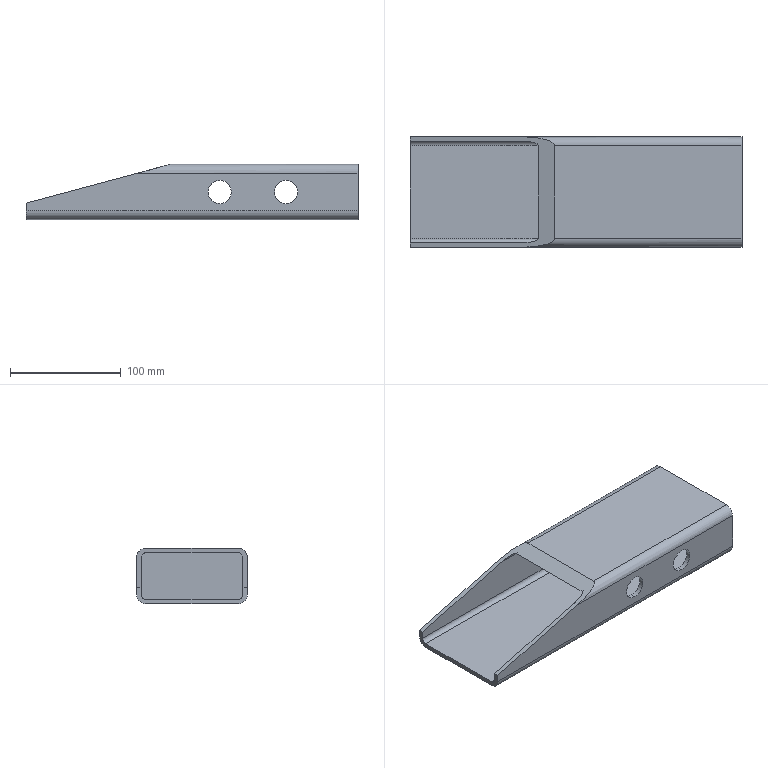Part | SolidWorks | features ICE 2, 3DProfileFeature 1, WeldMemberFeat 1, WeldmentFeature 1 | 2 solids | 37 faces | box 300 x 100 x 50 mm | volume 358178 mm3 | cylinder 20 | plane 17 | commonest cylinder face diameters 8 x8 21 x8 16 x4
STEP:
#1=CARTESIAN_POINT('',(235.,50.,-10.5));
#2=VERTEX_POINT('',#1);
#3=CARTESIAN_POINT('',(235.,50.,10.5));
#4=VERTEX_POINT('',#3);
#5=CARTESIAN_POINT('',(235.,50.,0.));
#6=DIRECTION('',(0.,1.,0.));
#7=DIRECTION('',(0.,0.,-1.));
#8=AXIS2_PLACEMENT_3D('',#5,#6,#7);
#9=CIRCLE('',#8,10.5);
#10=EDGE_CURVE('',#2,#4,#9,.T.);
#11=ORIENTED_EDGE('',*,*,#10,.T.);
#12=CARTESIAN_POINT('',(235.,46.,10.5));
#13=VERTEX_POINT('',#12);
#14=CARTESIAN_POINT('',(235.,185.23,10.5));
#15=DIRECTION('',(0.,-1.,0.));
#16=VECTOR('',#15,1000.);
#17=LINE('',#14,#16);
#18=EDGE_CURVE('',#4,#13,#17,.T.);
#19=ORIENTED_EDGE('',*,*,#18,.T.);
#20=CARTESIAN_POINT('',(235.,46.,-10.5));
#21=VERTEX_POINT('',#20);
#22=CARTESIAN_POINT('',(235.,46.,0.));
#23=DIRECTION('',(0.,-1.,0.));
#24=DIRECTION('',(0.,0.,-1.));
#25=AXIS2_PLACEMENT_3D('',#22,#23,#24);
#26=CIRCLE('',#25,10.5);
#27=EDGE_CURVE('',#13,#21,#26,.T.);
#28=ORIENTED_EDGE('',*,*,#27,.T.);
#29=CARTESIAN_POINT('',(235.,185.23,-10.5));
#30=DIRECTION('',(0.,-1.,0.));
#31=VECTOR('',#30,1000.);
#32=LINE('',#29,#31);
#33=EDGE_CURVE('',#2,#21,#32,.T.);
#34=ORIENTED_EDGE('',*,*,#33,.F.);
#35=EDGE_LOOP('',(#11,#19,#28,#34));
#36=FACE_OUTER_BOUND('',#35,.T.);
#37=CARTESIAN_POINT('',(235.,185.23,0.));
#38=DIRECTION('',(0.,-1.,0.));
#39=DIRECTION('',(0.,0.,-1.));
#40=AXIS2_PLACEMENT_3D('',#37,#38,#39);
#41=CYLINDRICAL_SURFACE('',#40,10.5);
#42=ADVANCED_FACE('',(#36),#41,.F.);
#43=CARTESIAN_POINT('',(175.,50.,-10.5));
#44=VERTEX_POINT('',#43);
#45=CARTESIAN_POINT('',(175.,50.,10.5));
#46=VERTEX_POINT('',#45);
#47=CARTESIAN_POINT('',(175.,50.,0.));
#48=DIRECTION('',(0.,1.,0.));
#49=DIRECTION('',(0.,0.,-1.));
#50=AXIS2_PLACEMENT_3D('',#47,#48,#49);
#51=CIRCLE('',#50,10.5);
#52=EDGE_CURVE('',#44,#46,#51,.T.);
#53=ORIENTED_EDGE('',*,*,#52,.T.);
#54=CARTESIAN_POINT('',(175.,46.,10.5));
#55=VERTEX_POINT('',#54);
#56=CARTESIAN_POINT('',(175.,185.23,10.5));
#57=DIRECTION('',(0.,-1.,0.));
#58=VECTOR('',#57,1000.);
#59=LINE('',#56,#58);
#60=EDGE_CURVE('',#46,#55,#59,.T.);
#61=ORIENTED_EDGE('',*,*,#60,.T.);
#62=CARTESIAN_POINT('',(175.,46.,-10.5));
#63=VERTEX_POINT('',#62);
#64=CARTESIAN_POINT('',(175.,46.,0.));
#65=DIRECTION('',(0.,-1.,0.));
#66=DIRECTION('',(0.,0.,-1.));
#67=AXIS2_PLACEMENT_3D('',#64,#65,#66);
#68=CIRCLE('',#67,10.5);
#69=EDGE_CURVE('',#55,#63,#68,.T.);
#70=ORIENTED_EDGE('',*,*,#69,.T.);
#71=CARTESIAN_POINT('',(175.,185.23,-10.5));
#72=DIRECTION('',(0.,-1.,0.));
#73=VECTOR('',#72,1000.);
#74=LINE('',#71,#73);
#75=EDGE_CURVE('',#44,#63,#74,.T.);
#76=ORIENTED_EDGE('',*,*,#75,.F.);
#77=EDGE_LOOP('',(#53,#61,#70,#76));
#78=FACE_OUTER_BOUND('',#77,.T.);
#79=CARTESIAN_POINT('',(175.,185.23,0.));
#80=DIRECTION('',(0.,-1.,0.));
#81=DIRECTION('',(0.,0.,-1.));
#82=AXIS2_PLACEMENT_3D('',#79,#80,#81);
#83=CYLINDRICAL_SURFACE('',#82,10.5);
#84=ADVANCED_FACE('',(#78),#83,.F.);
#85=CARTESIAN_POINT('',(235.,-46.,-10.5));
#86=VERTEX_POINT('',#85);
#87=CARTESIAN_POINT('',(235.,-46.,10.5));
#88=VERTEX_POINT('',#87);
#89=CARTESIAN_POINT('',(235.,-46.,0.));
#90=DIRECTION('',(0.,1.,0.));
#91=DIRECTION('',(0.,0.,1.));
#92=AXIS2_PLACEMENT_3D('',#89,#90,#91);
#93=CIRCLE('',#92,10.5);
#94=EDGE_CURVE('',#86,#88,#93,.T.);
#95=ORIENTED_EDGE('',*,*,#94,.T.);
#96=CARTESIAN_POINT('',(235.,-50.,10.5));
#97=VERTEX_POINT('',#96);
#98=CARTESIAN_POINT('',(235.,185.23,10.5));
#99=DIRECTION('',(0.,-1.,0.));
#100=VECTOR('',#99,1000.);
#101=LINE('',#98,#100);
#102=EDGE_CURVE('',#88,#97,#101,.T.);
#103=ORIENTED_EDGE('',*,*,#102,.T.);
#104=CARTESIAN_POINT('',(235.,-50.,-10.5));
#105=VERTEX_POINT('',#104);
#106=CARTESIAN_POINT('',(235.,-50.,0.));
#107=DIRECTION('',(0.,-1.,0.));
#108=DIRECTION('',(0.,0.,-1.));
#109=AXIS2_PLACEMENT_3D('',#106,#107,#108);
#110=CIRCLE('',#109,10.5);
#111=EDGE_CURVE('',#97,#105,#110,.T.);
#112=ORIENTED_EDGE('',*,*,#111,.T.);
#113=CARTESIAN_POINT('',(235.,185.23,-10.5));
#114=DIRECTION('',(0.,-1.,0.));
#115=VECTOR('',#114,1000.);
#116=LINE('',#113,#115);
#117=EDGE_CURVE('',#86,#105,#116,.T.);
#118=ORIENTED_EDGE('',*,*,#117,.F.);
#119=EDGE_LOOP('',(#95,#103,#112,#118));
#120=FACE_OUTER_BOUND('',#119,.T.);
#121=CARTESIAN_POINT('',(235.,185.23,0.));
#122=DIRECTION('',(0.,-1.,0.));
#123=DIRECTION('',(0.,0.,-1.));
#124=AXIS2_PLACEMENT_3D('',#121,#122,#123);
#125=CYLINDRICAL_SURFACE('',#124,10.5);
#126=ADVANCED_FACE('',(#120),#125,.F.);
#127=CARTESIAN_POINT('',(175.,-46.,-10.5));
#128=VERTEX_POINT('',#127);
#129=CARTESIAN_POINT('',(175.,-46.,10.5));
#130=VERTEX_POINT('',#129);
#131=CARTESIAN_POINT('',(175.,-46.,0.));
#132=DIRECTION('',(0.,1.,0.));
#133=DIRECTION('',(0.,0.,1.));
#134=AXIS2_PLACEMENT_3D('',#131,#132,#133);
#135=CIRCLE('',#134,10.5);
#136=EDGE_CURVE('',#128,#130,#135,.T.);
#137=ORIENTED_EDGE('',*,*,#136,.T.);
#138=CARTESIAN_POINT('',(175.,-50.,10.5));
#139=VERTEX_POINT('',#138);
#140=CARTESIAN_POINT('',(175.,185.23,10.5));
#141=DIRECTION('',(0.,-1.,0.));
#142=VECTOR('',#141,1000.);
#143=LINE('',#140,#142);
#144=EDGE_CURVE('',#130,#139,#143,.T.);
#145=ORIENTED_EDGE('',*,*,#144,.T.);
#146=CARTESIAN_POINT('',(175.,-50.,-10.5));
#147=VERTEX_POINT('',#146);
#148=CARTESIAN_POINT('',(175.,-50.,0.));
#149=DIRECTION('',(0.,-1.,0.));
#150=DIRECTION('',(0.,0.,-1.));
#151=AXIS2_PLACEMENT_3D('',#148,#149,#150);
#152=CIRCLE('',#151,10.5);
#153=EDGE_CURVE('',#139,#147,#152,.T.);
#154=ORIENTED_EDGE('',*,*,#153,.T.);
#155=CARTESIAN_POINT('',(175.,185.23,-10.5));
#156=DIRECTION('',(0.,-1.,0.));
#157=VECTOR('',#156,1000.);
#158=LINE('',#155,#157);
#159=EDGE_CURVE('',#128,#147,#158,.T.);
#160=ORIENTED_EDGE('',*,*,#159,.F.);
#161=EDGE_LOOP('',(#137,#145,#154,#160));
#162=FACE_OUTER_BOUND('',#161,.T.);
#163=CARTESIAN_POINT('',(175.,185.23,0.));
#164=DIRECTION('',(0.,-1.,0.));
#165=DIRECTION('',(0.,0.,-1.));
#166=AXIS2_PLACEMENT_3D('',#163,#164,#165);
#167=CYLINDRICAL_SURFACE('',#166,10.5);
#168=ADVANCED_FACE('',(#162),#167,.F.);
#169=CARTESIAN_POINT('',(0.,42.,-25.));
#170=VERTEX_POINT('',#169);
#171=CARTESIAN_POINT('',(0.,50.,-17.));
#172=VERTEX_POINT('',#171);
#173=CARTESIAN_POINT('',(0.,42.,-17.));
#174=DIRECTION('',(1.,0.,0.));
#175=DIRECTION('',(0.,0.,-1.));
#176=AXIS2_PLACEMENT_3D('',#173,#174,#175);
#177=CIRCLE('',#176,8.);
#178=EDGE_CURVE('',#170,#172,#177,.T.);
#179=ORIENTED_EDGE('',*,*,#178,.T.);
#180=CARTESIAN_POINT('',(300.,50.,-17.));
#181=VERTEX_POINT('',#180);
#182=CARTESIAN_POINT('',(300.,50.,-17.));
#183=DIRECTION('',(-1.,0.,0.));
#184=VECTOR('',#183,1000.);
#185=LINE('',#182,#184);
#186=EDGE_CURVE('',#181,#172,#185,.T.);
#187=ORIENTED_EDGE('',*,*,#186,.F.);
#188=CARTESIAN_POINT('',(300.,42.,-25.));
#189=VERTEX_POINT('',#188);
#190=CARTESIAN_POINT('',(300.,42.,-17.));
#191=DIRECTION('',(1.,0.,0.));
#192=DIRECTION('',(0.,0.,-1.));
#193=AXIS2_PLACEMENT_3D('',#190,#191,#192);
#194=CIRCLE('',#193,8.);
#195=EDGE_CURVE('',#189,#181,#194,.T.);
#196=ORIENTED_EDGE('',*,*,#195,.F.);
#197=CARTESIAN_POINT('',(300.,42.,-25.));
#198=DIRECTION('',(-1.,0.,0.));
#199=VECTOR('',#198,1000.);
#200=LINE('',#197,#199);
#201=EDGE_CURVE('',#189,#170,#200,.T.);
#202=ORIENTED_EDGE('',*,*,#201,.T.);
#203=EDGE_LOOP('',(#179,#187,#196,#202));
#204=FACE_OUTER_BOUND('',#203,.T.);
#205=CARTESIAN_POINT('',(300.,42.,-17.));
#206=DIRECTION('',(-1.,0.,0.));
#207=DIRECTION('',(0.,0.,1.));
#208=AXIS2_PLACEMENT_3D('',#205,#206,#207);
#209=CYLINDRICAL_SURFACE('',#208,8.);
#210=ADVANCED_FACE('',(#204),#209,.T.);
#211=ORIENTED_EDGE('',*,*,#10,.F.);
#212=CARTESIAN_POINT('',(235.,50.,0.));
#213=DIRECTION('',(0.,1.,0.));
#214=DIRECTION('',(0.,0.,-1.));
#215=AXIS2_PLACEMENT_3D('',#212,#213,#214);
#216=CIRCLE('',#215,10.5);
#217=EDGE_CURVE('',#4,#2,#216,.T.);
#218=ORIENTED_EDGE('',*,*,#217,.F.);
#219=EDGE_LOOP('',(#211,#218));
#220=FACE_BOUND('',#219,.T.);
#221=ORIENTED_EDGE('',*,*,#52,.F.);
#222=CARTESIAN_POINT('',(175.,50.,0.));
#223=DIRECTION('',(0.,1.,0.));
#224=DIRECTION('',(0.,0.,-1.));
#225=AXIS2_PLACEMENT_3D('',#222,#223,#224);
#226=CIRCLE('',#225,10.5);
#227=EDGE_CURVE('',#46,#44,#226,.T.);
#228=ORIENTED_EDGE('',*,*,#227,.F.);
#229=EDGE_LOOP('',(#221,#228));
#230=FACE_BOUND('',#229,.T.);
#231=CARTESIAN_POINT('',(0.,50.,-10.));
#232=VERTEX_POINT('',#231);
#233=CARTESIAN_POINT('',(0.,50.,-17.));
#234=DIRECTION('',(0.,0.,1.));
#235=VECTOR('',#234,1000.);
#236=LINE('',#233,#235);
#237=EDGE_CURVE('',#172,#232,#236,.T.);
#238=ORIENTED_EDGE('',*,*,#237,.T.);
#239=CARTESIAN_POINT('',(100.765,50.,17.));
#240=VERTEX_POINT('',#239);
#241=CARTESIAN_POINT('',(0.,50.,-10.));
#242=DIRECTION('',(-0.9659,0.,-0.2588));
#243=VECTOR('',#242,1000.);
#244=LINE('',#241,#243);
#245=EDGE_CURVE('',#240,#232,#244,.T.);
#246=ORIENTED_EDGE('',*,*,#245,.F.);
#247=CARTESIAN_POINT('',(300.,50.,17.));
#248=VERTEX_POINT('',#247);
#249=CARTESIAN_POINT('',(300.,50.,17.));
#250=DIRECTION('',(-1.,0.,0.));
#251=VECTOR('',#250,1000.);
#252=LINE('',#249,#251);
#253=EDGE_CURVE('',#248,#240,#252,.T.);
#254=ORIENTED_EDGE('',*,*,#253,.F.);
#255=CARTESIAN_POINT('',(300.,50.,-17.));
#256=DIRECTION('',(0.,0.,1.));
#257=VECTOR('',#256,1000.);
#258=LINE('',#255,#257);
#259=EDGE_CURVE('',#181,#248,#258,.T.);
#260=ORIENTED_EDGE('',*,*,#259,.F.);
#261=ORIENTED_EDGE('',*,*,#186,.T.);
#262=EDGE_LOOP('',(#238,#246,#254,#260,#261));
#263=FACE_OUTER_BOUND('',#262,.T.);
#264=CARTESIAN_POINT('',(300.,50.,-17.));
#265=DIRECTION('',(0.,-1.,0.));
#266=DIRECTION('',(0.,0.,-1.));
#267=AXIS2_PLACEMENT_3D('',#264,#265,#266);
#268=PLANE('',#267);
#269=ADVANCED_FACE('',(#220,#230,#263),#268,.F.);
#270=ORIENTED_EDGE('',*,*,#253,.T.);
#271=CARTESIAN_POINT('',(130.622,42.,25.));
#272=VERTEX_POINT('',#271);
#273=CARTESIAN_POINT('',(100.765,50.,17.));
#274=CARTESIAN_POINT('',(118.255,50.,21.686));
#275=CARTESIAN_POINT('',(130.622,46.686,25.));
#276=CARTESIAN_POINT('',(130.622,42.,25.));
#277=(BOUNDED_CURVE()B_SPLINE_CURVE(3,(#273,#274,#275,#276),.UNSPECIFIED.,.F.,.F.)B_SPLINE_CURVE_WITH_KNOTS((4,4),(1.571,3.142),.UNSPECIFIED.)CURVE()GEOMETRIC_REPRESENTATION_ITEM()RATIONAL_B_SPLINE_CURVE((1.,0.8047,0.8047,1.))REPRESENTATION_ITEM(''));
#278=EDGE_CURVE('',#240,#272,#277,.T.);
#279=ORIENTED_EDGE('',*,*,#278,.T.);
#280=CARTESIAN_POINT('',(300.,42.,25.));
#281=VERTEX_POINT('',#280);
#282=CARTESIAN_POINT('',(300.,42.,25.));
#283=DIRECTION('',(-1.,0.,0.));
#284=VECTOR('',#283,1000.);
#285=LINE('',#282,#284);
#286=EDGE_CURVE('',#281,#272,#285,.T.);
#287=ORIENTED_EDGE('',*,*,#286,.F.);
#288=CARTESIAN_POINT('',(300.,42.,17.));
#289=DIRECTION('',(1.,0.,0.));
#290=DIRECTION('',(0.,0.,-1.));
#291=AXIS2_PLACEMENT_3D('',#288,#289,#290);
#292=CIRCLE('',#291,8.);
#293=EDGE_CURVE('',#248,#281,#292,.T.);
#294=ORIENTED_EDGE('',*,*,#293,.F.);
#295=EDGE_LOOP('',(#270,#279,#287,#294));
#296=FACE_OUTER_BOUND('',#295,.T.);
#297=CARTESIAN_POINT('',(300.,42.,17.));
#298=DIRECTION('',(-1.,0.,0.));
#299=DIRECTION('',(0.,0.,1.));
#300=AXIS2_PLACEMENT_3D('',#297,#298,#299);
#301=CYLINDRICAL_SURFACE('',#300,8.);
#302=ADVANCED_FACE('',(#296),#301,.T.);
#303=ORIENTED_EDGE('',*,*,#286,.T.);
#304=CARTESIAN_POINT('',(130.622,-42.,25.));
#305=VERTEX_POINT('',#304);
#306=CARTESIAN_POINT('',(130.622,185.23,25.));
#307=DIRECTION('',(0.,-1.,0.));
#308=VECTOR('',#307,1000.);
#309=LINE('',#306,#308);
#310=EDGE_CURVE('',#272,#305,#309,.T.);
#311=ORIENTED_EDGE('',*,*,#310,.T.);
#312=CARTESIAN_POINT('',(300.,-42.,25.));
#313=VERTEX_POINT('',#312);
#314=CARTESIAN_POINT('',(300.,-42.,25.));
#315=DIRECTION('',(-1.,0.,0.));
#316=VECTOR('',#315,1000.);
#317=LINE('',#314,#316);
#318=EDGE_CURVE('',#313,#305,#317,.T.);
#319=ORIENTED_EDGE('',*,*,#318,.F.);
#320=CARTESIAN_POINT('',(300.,-42.,25.));
#321=DIRECTION('',(0.,-1.,0.));
#322=VECTOR('',#321,1000.);
#323=LINE('',#320,#322);
#324=EDGE_CURVE('',#281,#313,#323,.T.);
#325=ORIENTED_EDGE('',*,*,#324,.F.);
#326=EDGE_LOOP('',(#303,#311,#319,#325));
#327=FACE_OUTER_BOUND('',#326,.T.);
#328=CARTESIAN_POINT('',(300.,-42.,25.));
#329=DIRECTION('',(0.,0.,-1.));
#330=DIRECTION('',(-1.,0.,0.));
#331=AXIS2_PLACEMENT_3D('',#328,#329,#330);
#332=PLANE('',#331);
#333=ADVANCED_FACE('',(#327),#332,.F.);
#334=ORIENTED_EDGE('',*,*,#318,.T.);
#335=CARTESIAN_POINT('',(100.765,-50.,17.));
#336=VERTEX_POINT('',#335);
#337=CARTESIAN_POINT('',(130.622,-42.,25.));
#338=CARTESIAN_POINT('',(130.622,-46.686,25.));
#339=CARTESIAN_POINT('',(118.255,-50.,21.686));
#340=CARTESIAN_POINT('',(100.765,-50.,17.));
#341=(BOUNDED_CURVE()B_SPLINE_CURVE(3,(#337,#338,#339,#340),.UNSPECIFIED.,.F.,.F.)B_SPLINE_CURVE_WITH_KNOTS((4,4),(3.142,4.712),.UNSPECIFIED.)CURVE()GEOMETRIC_REPRESENTATION_ITEM()RATIONAL_B_SPLINE_CURVE((1.,0.8047,0.8047,1.))REPRESENTATION_ITEM(''));
#342=EDGE_CURVE('',#305,#336,#341,.T.);
#343=ORIENTED_EDGE('',*,*,#342,.T.);
#344=CARTESIAN_POINT('',(300.,-50.,17.));
#345=VERTEX_POINT('',#344);
#346=CARTESIAN_POINT('',(300.,-50.,17.));
#347=DIRECTION('',(-1.,0.,0.));
#348=VECTOR('',#347,1000.);
#349=LINE('',#346,#348);
#350=EDGE_CURVE('',#345,#336,#349,.T.);
#351=ORIENTED_EDGE('',*,*,#350,.F.);
#352=CARTESIAN_POINT('',(300.,-42.,17.));
#353=DIRECTION('',(1.,0.,0.));
#354=DIRECTION('',(0.,0.,-1.));
#355=AXIS2_PLACEMENT_3D('',#352,#353,#354);
#356=CIRCLE('',#355,8.);
#357=EDGE_CURVE('',#313,#345,#356,.T.);
#358=ORIENTED_EDGE('',*,*,#357,.F.);
#359=EDGE_LOOP('',(#334,#343,#351,#358));
#360=FACE_OUTER_BOUND('',#359,.T.);
#361=CARTESIAN_POINT('',(300.,-42.,17.));
#362=DIRECTION('',(-1.,0.,0.));
#363=DIRECTION('',(0.,0.,1.));
#364=AXIS2_PLACEMENT_3D('',#361,#362,#363);
#365=CYLINDRICAL_SURFACE('',#364,8.);
#366=ADVANCED_FACE('',(#360),#365,.T.);
#367=CARTESIAN_POINT('',(235.,-50.,0.));
#368=DIRECTION('',(0.,-1.,0.));
#369=DIRECTION('',(0.,0.,-1.));
#370=AXIS2_PLACEMENT_3D('',#367,#368,#369);
#371=CIRCLE('',#370,10.5);
#372=EDGE_CURVE('',#105,#97,#371,.T.);
#373=ORIENTED_EDGE('',*,*,#372,.F.);
#374=ORIENTED_EDGE('',*,*,#111,.F.);
#375=EDGE_LOOP('',(#373,#374));
#376=FACE_BOUND('',#375,.T.);
#377=CARTESIAN_POINT('',(175.,-50.,0.));
#378=DIRECTION('',(0.,-1.,0.));
#379=DIRECTION('',(0.,0.,-1.));
#380=AXIS2_PLACEMENT_3D('',#377,#378,#379);
#381=CIRCLE('',#380,10.5);
#382=EDGE_CURVE('',#147,#139,#381,.T.);
#383=ORIENTED_EDGE('',*,*,#382,.F.);
#384=ORIENTED_EDGE('',*,*,#153,.F.);
#385=EDGE_LOOP('',(#383,#384));
#386=FACE_BOUND('',#385,.T.);
#387=ORIENTED_EDGE('',*,*,#350,.T.);
#388=CARTESIAN_POINT('',(0.,-50.,-10.));
#389=VERTEX_POINT('',#388);
#390=CARTESIAN_POINT('',(0.,-50.,-10.));
#391=DIRECTION('',(0.9659,0.,0.2588));
#392=VECTOR('',#391,1000.);
#393=LINE('',#390,#392);
#394=EDGE_CURVE('',#389,#336,#393,.T.);
#395=ORIENTED_EDGE('',*,*,#394,.F.);
#396=CARTESIAN_POINT('',(0.,-50.,-17.));
#397=VERTEX_POINT('',#396);
#398=CARTESIAN_POINT('',(0.,-50.,17.));
#399=DIRECTION('',(0.,0.,-1.));
#400=VECTOR('',#399,1000.);
#401=LINE('',#398,#400);
#402=EDGE_CURVE('',#389,#397,#401,.T.);
#403=ORIENTED_EDGE('',*,*,#402,.T.);
#404=CARTESIAN_POINT('',(300.,-50.,-17.));
#405=VERTEX_POINT('',#404);
#406=CARTESIAN_POINT('',(300.,-50.,-17.));
#407=DIRECTION('',(-1.,0.,0.));
#408=VECTOR('',#407,1000.);
#409=LINE('',#406,#408);
#410=EDGE_CURVE('',#405,#397,#409,.T.);
#411=ORIENTED_EDGE('',*,*,#410,.F.);
#412=CARTESIAN_POINT('',(300.,-50.,17.));
#413=DIRECTION('',(0.,0.,-1.));
#414=VECTOR('',#413,1000.);
#415=LINE('',#412,#414);
#416=EDGE_CURVE('',#345,#405,#415,.T.);
#417=ORIENTED_EDGE('',*,*,#416,.F.);
#418=EDGE_LOOP('',(#387,#395,#403,#411,#417));
#419=FACE_OUTER_BOUND('',#418,.T.);
#420=CARTESIAN_POINT('',(300.,-50.,17.));
#421=DIRECTION('',(0.,1.,0.));
#422=DIRECTION('',(0.,0.,1.));
#423=AXIS2_PLACEMENT_3D('',#420,#421,#422);
#424=PLANE('',#423);
#425=ADVANCED_FACE('',(#376,#386,#419),#424,.F.);
#426=CARTESIAN_POINT('',(0.,-42.,-25.));
#427=VERTEX_POINT('',#426);
#428=CARTESIAN_POINT('',(0.,-42.,-17.));
#429=DIRECTION('',(1.,0.,0.));
#430=DIRECTION('',(0.,0.,-1.));
#431=AXIS2_PLACEMENT_3D('',#428,#429,#430);
#432=CIRCLE('',#431,8.);
#433=EDGE_CURVE('',#397,#427,#432,.T.);
#434=ORIENTED_EDGE('',*,*,#433,.T.);
#435=CARTESIAN_POINT('',(300.,-42.,-25.));
#436=VERTEX_POINT('',#435);
#437=CARTESIAN_POINT('',(300.,-42.,-25.));
#438=DIRECTION('',(-1.,0.,0.));
#439=VECTOR('',#438,1000.);
#440=LINE('',#437,#439);
#441=EDGE_CURVE('',#436,#427,#440,.T.);
#442=ORIENTED_EDGE('',*,*,#441,.F.);
#443=CARTESIAN_POINT('',(300.,-42.,-17.));
#444=DIRECTION('',(1.,0.,0.));
#445=DIRECTION('',(0.,0.,-1.));
#446=AXIS2_PLACEMENT_3D('',#443,#444,#445);
#447=CIRCLE('',#446,8.);
#448=EDGE_CURVE('',#405,#436,#447,.T.);
#449=ORIENTED_EDGE('',*,*,#448,.F.);
#450=ORIENTED_EDGE('',*,*,#410,.T.);
#451=EDGE_LOOP('',(#434,#442,#449,#450));
#452=FACE_OUTER_BOUND('',#451,.T.);
#453=CARTESIAN_POINT('',(300.,-42.,-17.));
#454=DIRECTION('',(-1.,0.,0.));
#455=DIRECTION('',(0.,0.,1.));
#456=AXIS2_PLACEMENT_3D('',#453,#454,#455);
#457=CYLINDRICAL_SURFACE('',#456,8.);
#458=ADVANCED_FACE('',(#452),#457,.T.);
#459=CARTESIAN_POINT('',(100.765,46.,17.));
#460=VERTEX_POINT('',#459);
#461=CARTESIAN_POINT('',(115.694,42.,21.));
#462=VERTEX_POINT('',#461);
#463=CARTESIAN_POINT('',(100.765,46.,17.));
#464=CARTESIAN_POINT('',(109.51,46.,19.343));
#465=CARTESIAN_POINT('',(115.694,44.343,21.));
#466=CARTESIAN_POINT('',(115.694,42.,21.));
#467=(BOUNDED_CURVE()B_SPLINE_CURVE(3,(#463,#464,#465,#466),.UNSPECIFIED.,.F.,.F.)B_SPLINE_CURVE_WITH_KNOTS((4,4),(1.571,3.142),.UNSPECIFIED.)CURVE()GEOMETRIC_REPRESENTATION_ITEM()RATIONAL_B_SPLINE_CURVE((1.,0.8047,0.8047,1.))REPRESENTATION_ITEM(''));
#468=EDGE_CURVE('',#460,#462,#467,.T.);
#469=ORIENTED_EDGE('',*,*,#468,.F.);
#470=CARTESIAN_POINT('',(300.,46.,17.));
#471=VERTEX_POINT('',#470);
#472=CARTESIAN_POINT('',(300.,46.,17.));
#473=DIRECTION('',(-1.,0.,0.));
#474=VECTOR('',#473,1000.);
#475=LINE('',#472,#474);
#476=EDGE_CURVE('',#471,#460,#475,.T.);
#477=ORIENTED_EDGE('',*,*,#476,.F.);
#478=CARTESIAN_POINT('',(300.,42.,21.));
#479=VERTEX_POINT('',#478);
#480=CARTESIAN_POINT('',(300.,42.,17.));
#481=DIRECTION('',(1.,0.,0.));
#482=DIRECTION('',(0.,0.,-1.));
#483=AXIS2_PLACEMENT_3D('',#480,#481,#482);
#484=CIRCLE('',#483,4.);
#485=EDGE_CURVE('',#471,#479,#484,.T.);
#486=ORIENTED_EDGE('',*,*,#485,.T.);
#487=CARTESIAN_POINT('',(300.,42.,21.));
#488=DIRECTION('',(-1.,0.,0.));
#489=VECTOR('',#488,1000.);
#490=LINE('',#487,#489);
#491=EDGE_CURVE('',#479,#462,#490,.T.);
#492=ORIENTED_EDGE('',*,*,#491,.T.);
#493=EDGE_LOOP('',(#469,#477,#486,#492));
#494=FACE_OUTER_BOUND('',#493,.T.);
#495=CARTESIAN_POINT('',(300.,42.,17.));
#496=DIRECTION('',(-1.,0.,0.));
#497=DIRECTION('',(0.,0.,1.));
#498=AXIS2_PLACEMENT_3D('',#495,#496,#497);
#499=CYLINDRICAL_SURFACE('',#498,4.);
#500=ADVANCED_FACE('',(#494),#499,.F.);
#501=CARTESIAN_POINT('',(235.,46.,0.));
#502=DIRECTION('',(0.,-1.,0.));
#503=DIRECTION('',(0.,0.,-1.));
#504=AXIS2_PLACEMENT_3D('',#501,#502,#503);
#505=CIRCLE('',#504,10.5);
#506=EDGE_CURVE('',#21,#13,#505,.T.);
#507=ORIENTED_EDGE('',*,*,#506,.F.);
#508=ORIENTED_EDGE('',*,*,#27,.F.);
#509=EDGE_LOOP('',(#507,#508));
#510=FACE_BOUND('',#509,.T.);
#511=CARTESIAN_POINT('',(175.,46.,0.));
#512=DIRECTION('',(0.,-1.,0.));
#513=DIRECTION('',(0.,0.,-1.));
#514=AXIS2_PLACEMENT_3D('',#511,#512,#513);
#515=CIRCLE('',#514,10.5);
#516=EDGE_CURVE('',#63,#55,#515,.T.);
#517=ORIENTED_EDGE('',*,*,#516,.F.);
#518=ORIENTED_EDGE('',*,*,#69,.F.);
#519=EDGE_LOOP('',(#517,#518));
#520=FACE_BOUND('',#519,.T.);
#521=CARTESIAN_POINT('',(0.,46.,-10.));
#522=VERTEX_POINT('',#521);
#523=CARTESIAN_POINT('',(278.154,46.,64.531));
#524=DIRECTION('',(0.9659,0.,0.2588));
#525=VECTOR('',#524,1000.);
#526=LINE('',#523,#525);
#527=EDGE_CURVE('',#522,#460,#526,.T.);
#528=ORIENTED_EDGE('',*,*,#527,.F.);
#529=CARTESIAN_POINT('',(0.,46.,-17.));
#530=VERTEX_POINT('',#529);
#531=CARTESIAN_POINT('',(0.,46.,-17.));
#532=DIRECTION('',(0.,0.,1.));
#533=VECTOR('',#532,1000.);
#534=LINE('',#531,#533);
#535=EDGE_CURVE('',#530,#522,#534,.T.);
#536=ORIENTED_EDGE('',*,*,#535,.F.);
#537=CARTESIAN_POINT('',(300.,46.,-17.));
#538=VERTEX_POINT('',#537);
#539=CARTESIAN_POINT('',(300.,46.,-17.));
#540=DIRECTION('',(-1.,0.,0.));
#541=VECTOR('',#540,1000.);
#542=LINE('',#539,#541);
#543=EDGE_CURVE('',#538,#530,#542,.T.);
#544=ORIENTED_EDGE('',*,*,#543,.F.);
#545=CARTESIAN_POINT('',(300.,46.,-17.));
#546=DIRECTION('',(0.,0.,1.));
#547=VECTOR('',#546,1000.);
#548=LINE('',#545,#547);
#549=EDGE_CURVE('',#538,#471,#548,.T.);
#550=ORIENTED_EDGE('',*,*,#549,.T.);
#551=ORIENTED_EDGE('',*,*,#476,.T.);
#552=EDGE_LOOP('',(#528,#536,#544,#550,#551));
#553=FACE_OUTER_BOUND('',#552,.T.);
#554=CARTESIAN_POINT('',(300.,46.,-17.));
#555=DIRECTION('',(0.,-1.,0.));
#556=DIRECTION('',(0.,0.,-1.));
#557=AXIS2_PLACEMENT_3D('',#554,#555,#556);
#558=PLANE('',#557);
#559=ADVANCED_FACE('',(#510,#520,#553),#558,.T.);
#560=CARTESIAN_POINT('',(0.,42.,-21.));
#561=VERTEX_POINT('',#560);
#562=CARTESIAN_POINT('',(0.,42.,-17.));
#563=DIRECTION('',(1.,0.,0.));
#564=DIRECTION('',(0.,0.,-1.));
#565=AXIS2_PLACEMENT_3D('',#562,#563,#564);
#566=CIRCLE('',#565,4.);
#567=EDGE_CURVE('',#561,#530,#566,.T.);
#568=ORIENTED_EDGE('',*,*,#567,.F.);
#569=CARTESIAN_POINT('',(300.,42.,-21.));
#570=VERTEX_POINT('',#569);
#571=CARTESIAN_POINT('',(300.,42.,-21.));
#572=DIRECTION('',(-1.,0.,0.));
#573=VECTOR('',#572,1000.);
#574=LINE('',#571,#573);
#575=EDGE_CURVE('',#570,#561,#574,.T.);
#576=ORIENTED_EDGE('',*,*,#575,.F.);
#577=CARTESIAN_POINT('',(300.,42.,-17.));
#578=DIRECTION('',(1.,0.,0.));
#579=DIRECTION('',(0.,0.,-1.));
#580=AXIS2_PLACEMENT_3D('',#577,#578,#579);
#581=CIRCLE('',#580,4.);
#582=EDGE_CURVE('',#570,#538,#581,.T.);
#583=ORIENTED_EDGE('',*,*,#582,.T.);
#584=ORIENTED_EDGE('',*,*,#543,.T.);
#585=EDGE_LOOP('',(#568,#576,#583,#584));
#586=FACE_OUTER_BOUND('',#585,.T.);
#587=CARTESIAN_POINT('',(300.,42.,-17.));
#588=DIRECTION('',(-1.,0.,0.));
#589=DIRECTION('',(0.,0.,1.));
#590=AXIS2_PLACEMENT_3D('',#587,#588,#589);
#591=CYLINDRICAL_SURFACE('',#590,4.);
#592=ADVANCED_FACE('',(#586),#591,.F.);
#593=CARTESIAN_POINT('',(0.,-42.,-21.));
#594=VERTEX_POINT('',#593);
#595=CARTESIAN_POINT('',(0.,42.,-21.));
#596=DIRECTION('',(0.,1.,0.));
#597=VECTOR('',#596,1000.);
#598=LINE('',#595,#597);
#599=EDGE_CURVE('',#594,#561,#598,.T.);
#600=ORIENTED_EDGE('',*,*,#599,.F.);
#601=CARTESIAN_POINT('',(300.,-42.,-21.));
#602=VERTEX_POINT('',#601);
#603=CARTESIAN_POINT('',(300.,-42.,-21.));
#604=DIRECTION('',(-1.,0.,0.));
#605=VECTOR('',#604,1000.);
#606=LINE('',#603,#605);
#607=EDGE_CURVE('',#602,#594,#606,.T.);
#608=ORIENTED_EDGE('',*,*,#607,.F.);
#609=CARTESIAN_POINT('',(300.,42.,-21.));
#610=DIRECTION('',(0.,1.,0.));
#611=VECTOR('',#610,1000.);
#612=LINE('',#609,#611);
#613=EDGE_CURVE('',#602,#570,#612,.T.);
#614=ORIENTED_EDGE('',*,*,#613,.T.);
#615=ORIENTED_EDGE('',*,*,#575,.T.);
#616=EDGE_LOOP('',(#600,#608,#614,#615));
#617=FACE_OUTER_BOUND('',#616,.T.);
#618=CARTESIAN_POINT('',(300.,42.,-21.));
#619=DIRECTION('',(0.,0.,1.));
#620=DIRECTION('',(1.,0.,0.));
#621=AXIS2_PLACEMENT_3D('',#618,#619,#620);
#622=PLANE('',#621);
#623=ADVANCED_FACE('',(#617),#622,.T.);
#624=CARTESIAN_POINT('',(0.,-46.,-17.));
#625=VERTEX_POINT('',#624);
#626=CARTESIAN_POINT('',(0.,-42.,-17.));
#627=DIRECTION('',(1.,0.,0.));
#628=DIRECTION('',(0.,0.,-1.));
#629=AXIS2_PLACEMENT_3D('',#626,#627,#628);
#630=CIRCLE('',#629,4.);
#631=EDGE_CURVE('',#625,#594,#630,.T.);
#632=ORIENTED_EDGE('',*,*,#631,.F.);
#633=CARTESIAN_POINT('',(300.,-46.,-17.));
#634=VERTEX_POINT('',#633);
#635=CARTESIAN_POINT('',(300.,-46.,-17.));
#636=DIRECTION('',(-1.,0.,0.));
#637=VECTOR('',#636,1000.);
#638=LINE('',#635,#637);
#639=EDGE_CURVE('',#634,#625,#638,.T.);
#640=ORIENTED_EDGE('',*,*,#639,.F.);
#641=CARTESIAN_POINT('',(300.,-42.,-17.));
#642=DIRECTION('',(1.,0.,0.));
#643=DIRECTION('',(0.,0.,-1.));
#644=AXIS2_PLACEMENT_3D('',#641,#642,#643);
#645=CIRCLE('',#644,4.);
#646=EDGE_CURVE('',#634,#602,#645,.T.);
#647=ORIENTED_EDGE('',*,*,#646,.T.);
#648=ORIENTED_EDGE('',*,*,#607,.T.);
#649=EDGE_LOOP('',(#632,#640,#647,#648));
#650=FACE_OUTER_BOUND('',#649,.T.);
#651=CARTESIAN_POINT('',(300.,-42.,-17.));
#652=DIRECTION('',(-1.,0.,0.));
#653=DIRECTION('',(0.,0.,1.));
#654=AXIS2_PLACEMENT_3D('',#651,#652,#653);
#655=CYLINDRICAL_SURFACE('',#654,4.);
#656=ADVANCED_FACE('',(#650),#655,.F.);
#657=ORIENTED_EDGE('',*,*,#94,.F.);
#658=CARTESIAN_POINT('',(235.,-46.,0.));
#659=DIRECTION('',(0.,1.,0.));
#660=DIRECTION('',(0.,0.,1.));
#661=AXIS2_PLACEMENT_3D('',#658,#659,#660);
#662=CIRCLE('',#661,10.5);
#663=EDGE_CURVE('',#88,#86,#662,.T.);
#664=ORIENTED_EDGE('',*,*,#663,.F.);
#665=EDGE_LOOP('',(#657,#664));
#666=FACE_BOUND('',#665,.T.);
#667=ORIENTED_EDGE('',*,*,#136,.F.);
#668=CARTESIAN_POINT('',(175.,-46.,0.));
#669=DIRECTION('',(0.,1.,0.));
#670=DIRECTION('',(0.,0.,1.));
#671=AXIS2_PLACEMENT_3D('',#668,#669,#670);
#672=CIRCLE('',#671,10.5);
#673=EDGE_CURVE('',#130,#128,#672,.T.);
#674=ORIENTED_EDGE('',*,*,#673,.F.);
#675=EDGE_LOOP('',(#667,#674));
#676=FACE_BOUND('',#675,.T.);
#677=CARTESIAN_POINT('',(100.765,-46.,17.));
#678=VERTEX_POINT('',#677);
#679=CARTESIAN_POINT('',(0.,-46.,-10.));
#680=VERTEX_POINT('',#679);
#681=CARTESIAN_POINT('',(286.654,-46.,66.809));
#682=DIRECTION('',(-0.9659,0.,-0.2588));
#683=VECTOR('',#682,1000.);
#684=LINE('',#681,#683);
#685=EDGE_CURVE('',#678,#680,#684,.T.);
#686=ORIENTED_EDGE('',*,*,#685,.F.);
#687=CARTESIAN_POINT('',(300.,-46.,17.));
#688=VERTEX_POINT('',#687);
#689=CARTESIAN_POINT('',(300.,-46.,17.));
#690=DIRECTION('',(-1.,0.,0.));
#691=VECTOR('',#690,1000.);
#692=LINE('',#689,#691);
#693=EDGE_CURVE('',#688,#678,#692,.T.);
#694=ORIENTED_EDGE('',*,*,#693,.F.);
#695=CARTESIAN_POINT('',(300.,-46.,17.));
#696=DIRECTION('',(0.,0.,-1.));
#697=VECTOR('',#696,1000.);
#698=LINE('',#695,#697);
#699=EDGE_CURVE('',#688,#634,#698,.T.);
#700=ORIENTED_EDGE('',*,*,#699,.T.);
#701=ORIENTED_EDGE('',*,*,#639,.T.);
#702=CARTESIAN_POINT('',(0.,-46.,17.));
#703=DIRECTION('',(0.,0.,-1.));
#704=VECTOR('',#703,1000.);
#705=LINE('',#702,#704);
#706=EDGE_CURVE('',#680,#625,#705,.T.);
#707=ORIENTED_EDGE('',*,*,#706,.F.);
#708=EDGE_LOOP('',(#686,#694,#700,#701,#707));
#709=FACE_OUTER_BOUND('',#708,.T.);
#710=CARTESIAN_POINT('',(300.,-46.,17.));
#711=DIRECTION('',(0.,1.,0.));
#712=DIRECTION('',(0.,0.,1.));
#713=AXIS2_PLACEMENT_3D('',#710,#711,#712);
#714=PLANE('',#713);
#715=ADVANCED_FACE('',(#666,#676,#709),#714,.T.);
#716=CARTESIAN_POINT('',(115.694,-42.,21.));
#717=VERTEX_POINT('',#716);
#718=CARTESIAN_POINT('',(115.694,-42.,21.));
#719=CARTESIAN_POINT('',(115.694,-44.343,21.));
#720=CARTESIAN_POINT('',(109.51,-46.,19.343));
#721=CARTESIAN_POINT('',(100.765,-46.,17.));
#722=(BOUNDED_CURVE()B_SPLINE_CURVE(3,(#718,#719,#720,#721),.UNSPECIFIED.,.F.,.F.)B_SPLINE_CURVE_WITH_KNOTS((4,4),(3.142,4.712),.UNSPECIFIED.)CURVE()GEOMETRIC_REPRESENTATION_ITEM()RATIONAL_B_SPLINE_CURVE((1.,0.8047,0.8047,1.))REPRESENTATION_ITEM(''));
#723=EDGE_CURVE('',#717,#678,#722,.T.);
#724=ORIENTED_EDGE('',*,*,#723,.F.);
#725=CARTESIAN_POINT('',(300.,-42.,21.));
#726=VERTEX_POINT('',#725);
#727=CARTESIAN_POINT('',(300.,-42.,21.));
#728=DIRECTION('',(-1.,0.,0.));
#729=VECTOR('',#728,1000.);
#730=LINE('',#727,#729);
#731=EDGE_CURVE('',#726,#717,#730,.T.);
#732=ORIENTED_EDGE('',*,*,#731,.F.);
#733=CARTESIAN_POINT('',(300.,-42.,17.));
#734=DIRECTION('',(1.,0.,0.));
#735=DIRECTION('',(0.,0.,-1.));
#736=AXIS2_PLACEMENT_3D('',#733,#734,#735);
#737=CIRCLE('',#736,4.);
#738=EDGE_CURVE('',#726,#688,#737,.T.);
#739=ORIENTED_EDGE('',*,*,#738,.T.);
#740=ORIENTED_EDGE('',*,*,#693,.T.);
#741=EDGE_LOOP('',(#724,#732,#739,#740));
#742=FACE_OUTER_BOUND('',#741,.T.);
#743=CARTESIAN_POINT('',(300.,-42.,17.));
#744=DIRECTION('',(-1.,0.,0.));
#745=DIRECTION('',(0.,0.,1.));
#746=AXIS2_PLACEMENT_3D('',#743,#744,#745);
#747=CYLINDRICAL_SURFACE('',#746,4.);
#748=ADVANCED_FACE('',(#742),#747,.F.);
#749=CARTESIAN_POINT('',(115.694,-42.,21.));
#750=DIRECTION('',(0.,-1.,0.));
#751=VECTOR('',#750,1000.);
#752=LINE('',#749,#751);
#753=EDGE_CURVE('',#462,#717,#752,.T.);
#754=ORIENTED_EDGE('',*,*,#753,.F.);
#755=ORIENTED_EDGE('',*,*,#491,.F.);
#756=CARTESIAN_POINT('',(300.,-42.,21.));
#757=DIRECTION('',(0.,-1.,0.));
#758=VECTOR('',#757,1000.);
#759=LINE('',#756,#758);
#760=EDGE_CURVE('',#479,#726,#759,.T.);
#761=ORIENTED_EDGE('',*,*,#760,.T.);
#762=ORIENTED_EDGE('',*,*,#731,.T.);
#763=EDGE_LOOP('',(#754,#755,#761,#762));
#764=FACE_OUTER_BOUND('',#763,.T.);
#765=CARTESIAN_POINT('',(300.,-42.,21.));
#766=DIRECTION('',(0.,0.,-1.));
#767=DIRECTION('',(-1.,0.,0.));
#768=AXIS2_PLACEMENT_3D('',#765,#766,#767);
#769=PLANE('',#768);
#770=ADVANCED_FACE('',(#764),#769,.T.);
#771=CARTESIAN_POINT('',(0.,42.,-25.));
#772=DIRECTION('',(0.,1.,0.));
#773=VECTOR('',#772,1000.);
#774=LINE('',#771,#773);
#775=EDGE_CURVE('',#427,#170,#774,.T.);
#776=ORIENTED_EDGE('',*,*,#775,.T.);
#777=ORIENTED_EDGE('',*,*,#201,.F.);
#778=CARTESIAN_POINT('',(300.,42.,-25.));
#779=DIRECTION('',(0.,1.,0.));
#780=VECTOR('',#779,1000.);
#781=LINE('',#778,#780);
#782=EDGE_CURVE('',#436,#189,#781,.T.);
#783=ORIENTED_EDGE('',*,*,#782,.F.);
#784=ORIENTED_EDGE('',*,*,#441,.T.);
#785=EDGE_LOOP('',(#776,#777,#783,#784));
#786=FACE_OUTER_BOUND('',#785,.T.);
#787=CARTESIAN_POINT('',(300.,42.,-25.));
#788=DIRECTION('',(0.,0.,1.));
#789=DIRECTION('',(1.,0.,0.));
#790=AXIS2_PLACEMENT_3D('',#787,#788,#789);
#791=PLANE('',#790);
#792=ADVANCED_FACE('',(#786),#791,.F.);
#793=ORIENTED_EDGE('',*,*,#485,.F.);
#794=ORIENTED_EDGE('',*,*,#549,.F.);
#795=ORIENTED_EDGE('',*,*,#582,.F.);
#796=ORIENTED_EDGE('',*,*,#613,.F.);
#797=ORIENTED_EDGE('',*,*,#646,.F.);
#798=ORIENTED_EDGE('',*,*,#699,.F.);
#799=ORIENTED_EDGE('',*,*,#738,.F.);
#800=ORIENTED_EDGE('',*,*,#760,.F.);
#801=EDGE_LOOP('',(#793,#794,#795,#796,#797,#798,#799,#800));
#802=FACE_BOUND('',#801,.T.);
#803=ORIENTED_EDGE('',*,*,#195,.T.);
#804=ORIENTED_EDGE('',*,*,#259,.T.);
#805=ORIENTED_EDGE('',*,*,#293,.T.);
#806=ORIENTED_EDGE('',*,*,#324,.T.);
#807=ORIENTED_EDGE('',*,*,#357,.T.);
#808=ORIENTED_EDGE('',*,*,#416,.T.);
#809=ORIENTED_EDGE('',*,*,#448,.T.);
#810=ORIENTED_EDGE('',*,*,#782,.T.);
#811=EDGE_LOOP('',(#803,#804,#805,#806,#807,#808,#809,#810));
#812=FACE_OUTER_BOUND('',#811,.T.);
#813=CARTESIAN_POINT('',(300.,42.,-17.));
#814=DIRECTION('',(1.,0.,0.));
#815=DIRECTION('',(0.,0.,-1.));
#816=AXIS2_PLACEMENT_3D('',#813,#814,#815);
#817=PLANE('',#816);
#818=ADVANCED_FACE('',(#802,#812),#817,.T.);
#819=ORIENTED_EDGE('',*,*,#402,.F.);
#820=CARTESIAN_POINT('',(0.,42.,-10.));
#821=DIRECTION('',(0.,1.,0.));
#822=VECTOR('',#821,1000.);
#823=LINE('',#820,#822);
#824=EDGE_CURVE('',#389,#680,#823,.T.);
#825=ORIENTED_EDGE('',*,*,#824,.T.);
#826=ORIENTED_EDGE('',*,*,#706,.T.);
#827=ORIENTED_EDGE('',*,*,#631,.T.);
#828=ORIENTED_EDGE('',*,*,#599,.T.);
#829=ORIENTED_EDGE('',*,*,#567,.T.);
#830=ORIENTED_EDGE('',*,*,#535,.T.);
#831=CARTESIAN_POINT('',(0.,185.23,-10.));
#832=DIRECTION('',(0.,-1.,0.));
#833=VECTOR('',#832,1000.);
#834=LINE('',#831,#833);
#835=EDGE_CURVE('',#232,#522,#834,.T.);
#836=ORIENTED_EDGE('',*,*,#835,.F.);
#837=ORIENTED_EDGE('',*,*,#237,.F.);
#838=ORIENTED_EDGE('',*,*,#178,.F.);
#839=ORIENTED_EDGE('',*,*,#775,.F.);
#840=ORIENTED_EDGE('',*,*,#433,.F.);
#841=EDGE_LOOP('',(#819,#825,#826,#827,#828,#829,#830,#836,#837,#838,#839,#840));
#842=FACE_OUTER_BOUND('',#841,.T.);
#843=CARTESIAN_POINT('',(0.,42.,-17.));
#844=DIRECTION('',(1.,0.,0.));
#845=DIRECTION('',(0.,0.,-1.));
#846=AXIS2_PLACEMENT_3D('',#843,#844,#845);
#847=PLANE('',#846);
#848=ADVANCED_FACE('',(#842),#847,.F.);
#849=ORIENTED_EDGE('',*,*,#245,.T.);
#850=ORIENTED_EDGE('',*,*,#835,.T.);
#851=ORIENTED_EDGE('',*,*,#527,.T.);
#852=ORIENTED_EDGE('',*,*,#468,.T.);
#853=ORIENTED_EDGE('',*,*,#753,.T.);
#854=ORIENTED_EDGE('',*,*,#723,.T.);
#855=ORIENTED_EDGE('',*,*,#685,.T.);
#856=ORIENTED_EDGE('',*,*,#824,.F.);
#857=ORIENTED_EDGE('',*,*,#394,.T.);
#858=ORIENTED_EDGE('',*,*,#342,.F.);
#859=ORIENTED_EDGE('',*,*,#310,.F.);
#860=ORIENTED_EDGE('',*,*,#278,.F.);
#861=EDGE_LOOP('',(#849,#850,#851,#852,#853,#854,#855,#856,#857,#858,#859,#860));
#862=FACE_OUTER_BOUND('',#861,.T.);
#863=CARTESIAN_POINT('',(0.,185.23,-10.));
#864=DIRECTION('',(0.2588,0.,-0.9659));
#865=DIRECTION('',(-0.9659,0.,-0.2588));
#866=AXIS2_PLACEMENT_3D('',#863,#864,#865);
#867=PLANE('',#866);
#868=ADVANCED_FACE('',(#862),#867,.F.);
#869=ORIENTED_EDGE('',*,*,#144,.F.);
#870=ORIENTED_EDGE('',*,*,#673,.T.);
#871=ORIENTED_EDGE('',*,*,#159,.T.);
#872=ORIENTED_EDGE('',*,*,#382,.T.);
#873=EDGE_LOOP('',(#869,#870,#871,#872));
#874=FACE_OUTER_BOUND('',#873,.T.);
#875=CARTESIAN_POINT('',(175.,185.23,0.));
#876=DIRECTION('',(0.,-1.,0.));
#877=DIRECTION('',(0.,0.,-1.));
#878=AXIS2_PLACEMENT_3D('',#875,#876,#877);
#879=CYLINDRICAL_SURFACE('',#878,10.5);
#880=ADVANCED_FACE('',(#874),#879,.F.);
#881=ORIENTED_EDGE('',*,*,#102,.F.);
#882=ORIENTED_EDGE('',*,*,#663,.T.);
#883=ORIENTED_EDGE('',*,*,#117,.T.);
#884=ORIENTED_EDGE('',*,*,#372,.T.);
#885=EDGE_LOOP('',(#881,#882,#883,#884));
#886=FACE_OUTER_BOUND('',#885,.T.);
#887=CARTESIAN_POINT('',(235.,185.23,0.));
#888=DIRECTION('',(0.,-1.,0.));
#889=DIRECTION('',(0.,0.,-1.));
#890=AXIS2_PLACEMENT_3D('',#887,#888,#889);
#891=CYLINDRICAL_SURFACE('',#890,10.5);
#892=ADVANCED_FACE('',(#886),#891,.F.);
#893=ORIENTED_EDGE('',*,*,#60,.F.);
#894=ORIENTED_EDGE('',*,*,#227,.T.);
#895=ORIENTED_EDGE('',*,*,#75,.T.);
#896=ORIENTED_EDGE('',*,*,#516,.T.);
#897=EDGE_LOOP('',(#893,#894,#895,#896));
#898=FACE_OUTER_BOUND('',#897,.T.);
#899=CARTESIAN_POINT('',(175.,185.23,0.));
#900=DIRECTION('',(0.,-1.,0.));
#901=DIRECTION('',(0.,0.,-1.));
#902=AXIS2_PLACEMENT_3D('',#899,#900,#901);
#903=CYLINDRICAL_SURFACE('',#902,10.5);
#904=ADVANCED_FACE('',(#898),#903,.F.);
#905=ORIENTED_EDGE('',*,*,#18,.F.);
#906=ORIENTED_EDGE('',*,*,#217,.T.);
#907=ORIENTED_EDGE('',*,*,#33,.T.);
#908=ORIENTED_EDGE('',*,*,#506,.T.);
#909=EDGE_LOOP('',(#905,#906,#907,#908));
#910=FACE_OUTER_BOUND('',#909,.T.);
#911=CARTESIAN_POINT('',(235.,185.23,0.));
#912=DIRECTION('',(0.,-1.,0.));
#913=DIRECTION('',(0.,0.,-1.));
#914=AXIS2_PLACEMENT_3D('',#911,#912,#913);
#915=CYLINDRICAL_SURFACE('',#914,10.5);
#916=ADVANCED_FACE('',(#910),#915,.F.);
#917=CLOSED_SHELL('',(#42,#84,#126,#168,#210,#269,#302,#333,#366,#425,#458,#500,#559,#592,#623,#656,#715,#748,#770,#792,#818,#848,#868,#880,#892,#904,#916));
#918=MANIFOLD_SOLID_BREP('',#917);
#919=CARTESIAN_POINT('',(300.,-42.,21.));
#920=VERTEX_POINT('',#919);
#921=CARTESIAN_POINT('',(300.,-46.,17.));
#922=VERTEX_POINT('',#921);
#923=CARTESIAN_POINT('',(300.,-42.,17.));
#924=DIRECTION('',(1.,0.,0.));
#925=DIRECTION('',(0.,0.,-1.));
#926=AXIS2_PLACEMENT_3D('',#923,#924,#925);
#927=CIRCLE('',#926,4.);
#928=EDGE_CURVE('',#920,#922,#927,.T.);
#929=ORIENTED_EDGE('',*,*,#928,.F.);
#930=CARTESIAN_POINT('',(275.,-42.,21.));
#931=VERTEX_POINT('',#930);
#932=CARTESIAN_POINT('',(275.,-42.,21.));
#933=DIRECTION('',(1.,0.,0.));
#934=VECTOR('',#933,1000.);
#935=LINE('',#932,#934);
#936=EDGE_CURVE('',#931,#920,#935,.T.);
#937=ORIENTED_EDGE('',*,*,#936,.F.);
#938=CARTESIAN_POINT('',(275.,-46.,17.));
#939=VERTEX_POINT('',#938);
#940=CARTESIAN_POINT('',(275.,-42.,17.));
#941=DIRECTION('',(1.,0.,0.));
#942=DIRECTION('',(0.,0.,-1.));
#943=AXIS2_PLACEMENT_3D('',#940,#941,#942);
#944=CIRCLE('',#943,4.);
#945=EDGE_CURVE('',#931,#939,#944,.T.);
#946=ORIENTED_EDGE('',*,*,#945,.T.);
#947=CARTESIAN_POINT('',(275.,-46.,17.));
#948=DIRECTION('',(1.,0.,0.));
#949=VECTOR('',#948,1000.);
#950=LINE('',#947,#949);
#951=EDGE_CURVE('',#939,#922,#950,.T.);
#952=ORIENTED_EDGE('',*,*,#951,.T.);
#953=EDGE_LOOP('',(#929,#937,#946,#952));
#954=FACE_OUTER_BOUND('',#953,.T.);
#955=CARTESIAN_POINT('',(275.,-42.,17.));
#956=DIRECTION('',(1.,0.,0.));
#957=DIRECTION('',(0.,0.,-1.));
#958=AXIS2_PLACEMENT_3D('',#955,#956,#957);
#959=CYLINDRICAL_SURFACE('',#958,4.);
#960=ADVANCED_FACE('',(#954),#959,.T.);
#961=CARTESIAN_POINT('',(300.,42.,21.));
#962=VERTEX_POINT('',#961);
#963=CARTESIAN_POINT('',(300.,42.,21.));
#964=DIRECTION('',(0.,-1.,0.));
#965=VECTOR('',#964,1000.);
#966=LINE('',#963,#965);
#967=EDGE_CURVE('',#962,#920,#966,.T.);
#968=ORIENTED_EDGE('',*,*,#967,.F.);
#969=CARTESIAN_POINT('',(275.,42.,21.));
#970=VERTEX_POINT('',#969);
#971=CARTESIAN_POINT('',(275.,42.,21.));
#972=DIRECTION('',(1.,0.,0.));
#973=VECTOR('',#972,1000.);
#974=LINE('',#971,#973);
#975=EDGE_CURVE('',#970,#962,#974,.T.);
#976=ORIENTED_EDGE('',*,*,#975,.F.);
#977=CARTESIAN_POINT('',(275.,42.,21.));
#978=DIRECTION('',(0.,-1.,0.));
#979=VECTOR('',#978,1000.);
#980=LINE('',#977,#979);
#981=EDGE_CURVE('',#970,#931,#980,.T.);
#982=ORIENTED_EDGE('',*,*,#981,.T.);
#983=ORIENTED_EDGE('',*,*,#936,.T.);
#984=EDGE_LOOP('',(#968,#976,#982,#983));
#985=FACE_OUTER_BOUND('',#984,.T.);
#986=CARTESIAN_POINT('',(275.,42.,21.));
#987=DIRECTION('',(0.,0.,1.));
#988=DIRECTION('',(0.,-1.,0.));
#989=AXIS2_PLACEMENT_3D('',#986,#987,#988);
#990=PLANE('',#989);
#991=ADVANCED_FACE('',(#985),#990,.T.);
#992=CARTESIAN_POINT('',(300.,46.,17.));
#993=VERTEX_POINT('',#992);
#994=CARTESIAN_POINT('',(300.,42.,17.));
#995=DIRECTION('',(1.,0.,0.));
#996=DIRECTION('',(0.,0.,-1.));
#997=AXIS2_PLACEMENT_3D('',#994,#995,#996);
#998=CIRCLE('',#997,4.);
#999=EDGE_CURVE('',#993,#962,#998,.T.);
#1000=ORIENTED_EDGE('',*,*,#999,.F.);
#1001=CARTESIAN_POINT('',(275.,46.,17.));
#1002=VERTEX_POINT('',#1001);
#1003=CARTESIAN_POINT('',(275.,46.,17.));
#1004=DIRECTION('',(1.,0.,0.));
#1005=VECTOR('',#1004,1000.);
#1006=LINE('',#1003,#1005);
#1007=EDGE_CURVE('',#1002,#993,#1006,.T.);
#1008=ORIENTED_EDGE('',*,*,#1007,.F.);
#1009=CARTESIAN_POINT('',(275.,42.,17.));
#1010=DIRECTION('',(1.,0.,0.));
#1011=DIRECTION('',(0.,0.,-1.));
#1012=AXIS2_PLACEMENT_3D('',#1009,#1010,#1011);
#1013=CIRCLE('',#1012,4.);
#1014=EDGE_CURVE('',#1002,#970,#1013,.T.);
#1015=ORIENTED_EDGE('',*,*,#1014,.T.);
#1016=ORIENTED_EDGE('',*,*,#975,.T.);
#1017=EDGE_LOOP('',(#1000,#1008,#1015,#1016));
#1018=FACE_OUTER_BOUND('',#1017,.T.);
#1019=CARTESIAN_POINT('',(275.,42.,17.));
#1020=DIRECTION('',(1.,0.,0.));
#1021=DIRECTION('',(0.,0.,-1.));
#1022=AXIS2_PLACEMENT_3D('',#1019,#1020,#1021);
#1023=CYLINDRICAL_SURFACE('',#1022,4.);
#1024=ADVANCED_FACE('',(#1018),#1023,.T.);
#1025=CARTESIAN_POINT('',(300.,46.,-17.));
#1026=VERTEX_POINT('',#1025);
#1027=CARTESIAN_POINT('',(300.,46.,17.));
#1028=DIRECTION('',(0.,0.,1.));
#1029=VECTOR('',#1028,1000.);
#1030=LINE('',#1027,#1029);
#1031=EDGE_CURVE('',#1026,#993,#1030,.T.);
#1032=ORIENTED_EDGE('',*,*,#1031,.F.);
#1033=CARTESIAN_POINT('',(275.,46.,-17.));
#1034=VERTEX_POINT('',#1033);
#1035=CARTESIAN_POINT('',(275.,46.,-17.));
#1036=DIRECTION('',(1.,0.,0.));
#1037=VECTOR('',#1036,1000.);
#1038=LINE('',#1035,#1037);
#1039=EDGE_CURVE('',#1034,#1026,#1038,.T.);
#1040=ORIENTED_EDGE('',*,*,#1039,.F.);
#1041=CARTESIAN_POINT('',(275.,46.,17.));
#1042=DIRECTION('',(0.,0.,1.));
#1043=VECTOR('',#1042,1000.);
#1044=LINE('',#1041,#1043);
#1045=EDGE_CURVE('',#1034,#1002,#1044,.T.);
#1046=ORIENTED_EDGE('',*,*,#1045,.T.);
#1047=ORIENTED_EDGE('',*,*,#1007,.T.);
#1048=EDGE_LOOP('',(#1032,#1040,#1046,#1047));
#1049=FACE_OUTER_BOUND('',#1048,.T.);
#1050=CARTESIAN_POINT('',(275.,46.,17.));
#1051=DIRECTION('',(0.,1.,0.));
#1052=DIRECTION('',(0.,0.,1.));
#1053=AXIS2_PLACEMENT_3D('',#1050,#1051,#1052);
#1054=PLANE('',#1053);
#1055=ADVANCED_FACE('',(#1049),#1054,.T.);
#1056=CARTESIAN_POINT('',(300.,42.,-21.));
#1057=VERTEX_POINT('',#1056);
#1058=CARTESIAN_POINT('',(300.,42.,-17.));
#1059=DIRECTION('',(1.,0.,0.));
#1060=DIRECTION('',(0.,0.,1.));
#1061=AXIS2_PLACEMENT_3D('',#1058,#1059,#1060);
#1062=CIRCLE('',#1061,4.);
#1063=EDGE_CURVE('',#1057,#1026,#1062,.T.);
#1064=ORIENTED_EDGE('',*,*,#1063,.F.);
#1065=CARTESIAN_POINT('',(275.,42.,-21.));
#1066=VERTEX_POINT('',#1065);
#1067=CARTESIAN_POINT('',(275.,42.,-21.));
#1068=DIRECTION('',(1.,0.,0.));
#1069=VECTOR('',#1068,1000.);
#1070=LINE('',#1067,#1069);
#1071=EDGE_CURVE('',#1066,#1057,#1070,.T.);
#1072=ORIENTED_EDGE('',*,*,#1071,.F.);
#1073=CARTESIAN_POINT('',(275.,42.,-17.));
#1074=DIRECTION('',(1.,0.,0.));
#1075=DIRECTION('',(0.,0.,1.));
#1076=AXIS2_PLACEMENT_3D('',#1073,#1074,#1075);
#1077=CIRCLE('',#1076,4.);
#1078=EDGE_CURVE('',#1066,#1034,#1077,.T.);
#1079=ORIENTED_EDGE('',*,*,#1078,.T.);
#1080=ORIENTED_EDGE('',*,*,#1039,.T.);
#1081=EDGE_LOOP('',(#1064,#1072,#1079,#1080));
#1082=FACE_OUTER_BOUND('',#1081,.T.);
#1083=CARTESIAN_POINT('',(275.,42.,-17.));
#1084=DIRECTION('',(1.,0.,0.));
#1085=DIRECTION('',(0.,0.,-1.));
#1086=AXIS2_PLACEMENT_3D('',#1083,#1084,#1085);
#1087=CYLINDRICAL_SURFACE('',#1086,4.);
#1088=ADVANCED_FACE('',(#1082),#1087,.T.);
#1089=CARTESIAN_POINT('',(300.,-42.,-21.));
#1090=VERTEX_POINT('',#1089);
#1091=CARTESIAN_POINT('',(300.,42.,-21.));
#1092=DIRECTION('',(0.,1.,0.));
#1093=VECTOR('',#1092,1000.);
#1094=LINE('',#1091,#1093);
#1095=EDGE_CURVE('',#1090,#1057,#1094,.T.);
#1096=ORIENTED_EDGE('',*,*,#1095,.F.);
#1097=CARTESIAN_POINT('',(275.,-42.,-21.));
#1098=VERTEX_POINT('',#1097);
#1099=CARTESIAN_POINT('',(275.,-42.,-21.));
#1100=DIRECTION('',(1.,0.,0.));
#1101=VECTOR('',#1100,1000.);
#1102=LINE('',#1099,#1101);
#1103=EDGE_CURVE('',#1098,#1090,#1102,.T.);
#1104=ORIENTED_EDGE('',*,*,#1103,.F.);
#1105=CARTESIAN_POINT('',(275.,42.,-21.));
#1106=DIRECTION('',(0.,1.,0.));
#1107=VECTOR('',#1106,1000.);
#1108=LINE('',#1105,#1107);
#1109=EDGE_CURVE('',#1098,#1066,#1108,.T.);
#1110=ORIENTED_EDGE('',*,*,#1109,.T.);
#1111=ORIENTED_EDGE('',*,*,#1071,.T.);
#1112=EDGE_LOOP('',(#1096,#1104,#1110,#1111));
#1113=FACE_OUTER_BOUND('',#1112,.T.);
#1114=CARTESIAN_POINT('',(275.,42.,-21.));
#1115=DIRECTION('',(0.,0.,-1.));
#1116=DIRECTION('',(0.,1.,0.));
#1117=AXIS2_PLACEMENT_3D('',#1114,#1115,#1116);
#1118=PLANE('',#1117);
#1119=ADVANCED_FACE('',(#1113),#1118,.T.);
#1120=CARTESIAN_POINT('',(300.,-46.,-17.));
#1121=VERTEX_POINT('',#1120);
#1122=CARTESIAN_POINT('',(300.,-42.,-17.));
#1123=DIRECTION('',(1.,0.,0.));
#1124=DIRECTION('',(0.,0.,-1.));
#1125=AXIS2_PLACEMENT_3D('',#1122,#1123,#1124);
#1126=CIRCLE('',#1125,4.);
#1127=EDGE_CURVE('',#1121,#1090,#1126,.T.);
#1128=ORIENTED_EDGE('',*,*,#1127,.F.);
#1129=CARTESIAN_POINT('',(275.,-46.,-17.));
#1130=VERTEX_POINT('',#1129);
#1131=CARTESIAN_POINT('',(275.,-46.,-17.));
#1132=DIRECTION('',(1.,0.,0.));
#1133=VECTOR('',#1132,1000.);
#1134=LINE('',#1131,#1133);
#1135=EDGE_CURVE('',#1130,#1121,#1134,.T.);
#1136=ORIENTED_EDGE('',*,*,#1135,.F.);
#1137=CARTESIAN_POINT('',(275.,-42.,-17.));
#1138=DIRECTION('',(1.,0.,0.));
#1139=DIRECTION('',(0.,0.,-1.));
#1140=AXIS2_PLACEMENT_3D('',#1137,#1138,#1139);
#1141=CIRCLE('',#1140,4.);
#1142=EDGE_CURVE('',#1130,#1098,#1141,.T.);
#1143=ORIENTED_EDGE('',*,*,#1142,.T.);
#1144=ORIENTED_EDGE('',*,*,#1103,.T.);
#1145=EDGE_LOOP('',(#1128,#1136,#1143,#1144));
#1146=FACE_OUTER_BOUND('',#1145,.T.);
#1147=CARTESIAN_POINT('',(275.,-42.,-17.));
#1148=DIRECTION('',(1.,0.,0.));
#1149=DIRECTION('',(0.,0.,-1.));
#1150=AXIS2_PLACEMENT_3D('',#1147,#1148,#1149);
#1151=CYLINDRICAL_SURFACE('',#1150,4.);
#1152=ADVANCED_FACE('',(#1146),#1151,.T.);
#1153=CARTESIAN_POINT('',(300.,-46.,17.));
#1154=DIRECTION('',(0.,0.,-1.));
#1155=VECTOR('',#1154,1000.);
#1156=LINE('',#1153,#1155);
#1157=EDGE_CURVE('',#922,#1121,#1156,.T.);
#1158=ORIENTED_EDGE('',*,*,#1157,.F.);
#1159=ORIENTED_EDGE('',*,*,#951,.F.);
#1160=CARTESIAN_POINT('',(275.,-46.,17.));
#1161=DIRECTION('',(0.,0.,-1.));
#1162=VECTOR('',#1161,1000.);
#1163=LINE('',#1160,#1162);
#1164=EDGE_CURVE('',#939,#1130,#1163,.T.);
#1165=ORIENTED_EDGE('',*,*,#1164,.T.);
#1166=ORIENTED_EDGE('',*,*,#1135,.T.);
#1167=EDGE_LOOP('',(#1158,#1159,#1165,#1166));
#1168=FACE_OUTER_BOUND('',#1167,.T.);
#1169=CARTESIAN_POINT('',(275.,-46.,17.));
#1170=DIRECTION('',(0.,-1.,0.));
#1171=DIRECTION('',(0.,0.,-1.));
#1172=AXIS2_PLACEMENT_3D('',#1169,#1170,#1171);
#1173=PLANE('',#1172);
#1174=ADVANCED_FACE('',(#1168),#1173,.T.);
#1175=ORIENTED_EDGE('',*,*,#945,.F.);
#1176=ORIENTED_EDGE('',*,*,#981,.F.);
#1177=ORIENTED_EDGE('',*,*,#1014,.F.);
#1178=ORIENTED_EDGE('',*,*,#1045,.F.);
#1179=ORIENTED_EDGE('',*,*,#1078,.F.);
#1180=ORIENTED_EDGE('',*,*,#1109,.F.);
#1181=ORIENTED_EDGE('',*,*,#1142,.F.);
#1182=ORIENTED_EDGE('',*,*,#1164,.F.);
#1183=EDGE_LOOP('',(#1175,#1176,#1177,#1178,#1179,#1180,#1181,#1182));
#1184=FACE_OUTER_BOUND('',#1183,.T.);
#1185=CARTESIAN_POINT('',(275.,-42.,17.));
#1186=DIRECTION('',(1.,0.,0.));
#1187=DIRECTION('',(0.,0.,-1.));
#1188=AXIS2_PLACEMENT_3D('',#1185,#1186,#1187);
#1189=PLANE('',#1188);
#1190=ADVANCED_FACE('',(#1184),#1189,.F.);
#1191=ORIENTED_EDGE('',*,*,#928,.T.);
#1192=ORIENTED_EDGE('',*,*,#1157,.T.);
#1193=ORIENTED_EDGE('',*,*,#1127,.T.);
#1194=ORIENTED_EDGE('',*,*,#1095,.T.);
#1195=ORIENTED_EDGE('',*,*,#1063,.T.);
#1196=ORIENTED_EDGE('',*,*,#1031,.T.);
#1197=ORIENTED_EDGE('',*,*,#999,.T.);
#1198=ORIENTED_EDGE('',*,*,#967,.T.);
#1199=EDGE_LOOP('',(#1191,#1192,#1193,#1194,#1195,#1196,#1197,#1198));
#1200=FACE_OUTER_BOUND('',#1199,.T.);
#1201=CARTESIAN_POINT('',(300.,-42.,17.));
#1202=DIRECTION('',(1.,0.,0.));
#1203=DIRECTION('',(0.,0.,-1.));
#1204=AXIS2_PLACEMENT_3D('',#1201,#1202,#1203);
#1205=PLANE('',#1204);
#1206=ADVANCED_FACE('',(#1200),#1205,.T.);
#1207=CLOSED_SHELL('',(#960,#991,#1024,#1055,#1088,#1119,#1152,#1174,#1190,#1206));
#1208=MANIFOLD_SOLID_BREP('',#1207);
#1209=CARTESIAN_POINT('',(0.,0.,0.));
#1210=DIRECTION('',(0.,0.,1.));
#1211=DIRECTION('',(1.,0.,0.));
#1212=AXIS2_PLACEMENT_3D('',#1209,#1210,#1211);
#1213=(LENGTH_UNIT()NAMED_UNIT(*)SI_UNIT(.MILLI.,.METRE.));
#1214=UNCERTAINTY_MEASURE_WITH_UNIT(LENGTH_MEASURE(0.00001),#1213,'','');
#1215=(NAMED_UNIT(*)PLANE_ANGLE_UNIT()SI_UNIT($,.RADIAN.));
#1216=(NAMED_UNIT(*)SI_UNIT($,.STERADIAN.)SOLID_ANGLE_UNIT());
#1217=(GEOMETRIC_REPRESENTATION_CONTEXT(3)GLOBAL_UNCERTAINTY_ASSIGNED_CONTEXT((#1214))GLOBAL_UNIT_ASSIGNED_CONTEXT((#1213,#1215,#1216))REPRESENTATION_CONTEXT('',''));
#1218=ADVANCED_BREP_SHAPE_REPRESENTATION('',(#918,#1208,#1212),#1217);